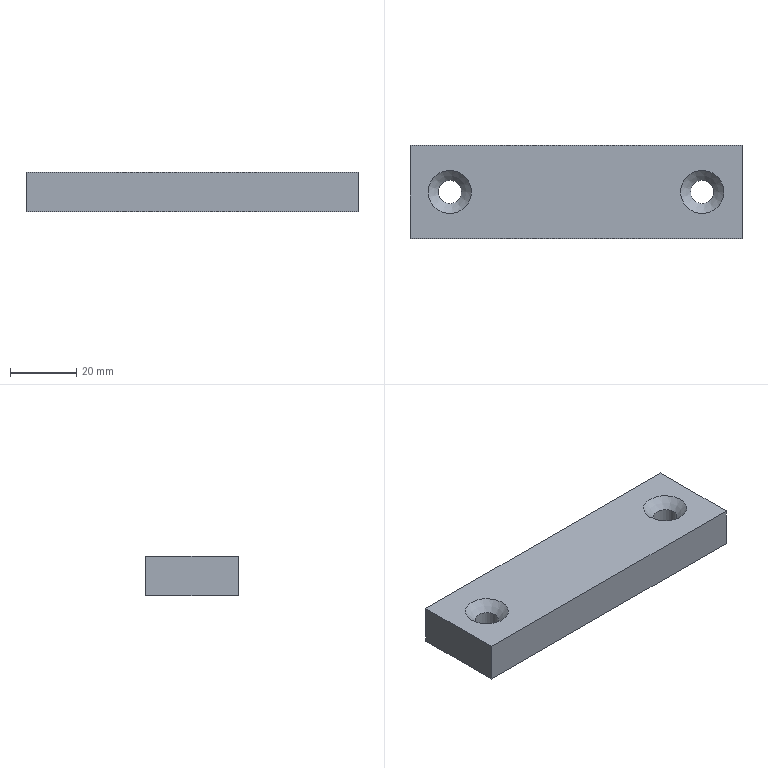Part | NX | features DATUM_CSYS 2, CHAMFER 1, EXTRUDE 1, SKETCH 1 | 1 solid | 10 faces | box 100 x 28 x 12 mm | volume 32422 mm3 | plane 6 | cylinder 2 | cone 2 | commonest cylinder face diameters 7 x2
STEP:
#1=CARTESIAN_POINT('',(-50.,-14.,0.));
#2=VERTEX_POINT('',#1);
#3=CARTESIAN_POINT('',(-50.,14.,0.));
#4=VERTEX_POINT('',#3);
#5=CARTESIAN_POINT('',(-50.,-14.,0.));
#6=DIRECTION('',(0.,1.,0.));
#7=VECTOR('',#6,1000.);
#8=LINE('',#5,#7);
#9=EDGE_CURVE('',#2,#4,#8,.T.);
#10=ORIENTED_EDGE('',*,*,#9,.T.);
#11=CARTESIAN_POINT('',(-50.,14.,-12.));
#12=VERTEX_POINT('',#11);
#13=CARTESIAN_POINT('',(-50.,14.,-12.));
#14=DIRECTION('',(0.,0.,1.));
#15=VECTOR('',#14,1000.);
#16=LINE('',#13,#15);
#17=EDGE_CURVE('',#12,#4,#16,.T.);
#18=ORIENTED_EDGE('',*,*,#17,.F.);
#19=CARTESIAN_POINT('',(-50.,-14.,-12.));
#20=VERTEX_POINT('',#19);
#21=CARTESIAN_POINT('',(-50.,-14.,-12.));
#22=DIRECTION('',(0.,1.,0.));
#23=VECTOR('',#22,1000.);
#24=LINE('',#21,#23);
#25=EDGE_CURVE('',#20,#12,#24,.T.);
#26=ORIENTED_EDGE('',*,*,#25,.F.);
#27=CARTESIAN_POINT('',(-50.,-14.,-12.));
#28=DIRECTION('',(0.,0.,1.));
#29=VECTOR('',#28,1000.);
#30=LINE('',#27,#29);
#31=EDGE_CURVE('',#20,#2,#30,.T.);
#32=ORIENTED_EDGE('',*,*,#31,.T.);
#33=EDGE_LOOP('',(#10,#18,#26,#32));
#34=FACE_BOUND('',#33,.T.);
#35=CARTESIAN_POINT('',(-50.,-14.,-12.));
#36=DIRECTION('',(1.,0.,0.));
#37=DIRECTION('',(0.,0.,-1.));
#38=AXIS2_PLACEMENT_3D('',#35,#36,#37);
#39=PLANE('',#38);
#40=ADVANCED_FACE('',(#34),#39,.F.);
#41=CARTESIAN_POINT('',(50.,14.,0.));
#42=VERTEX_POINT('',#41);
#43=CARTESIAN_POINT('',(-50.,14.,0.));
#44=DIRECTION('',(1.,0.,0.));
#45=VECTOR('',#44,1000.);
#46=LINE('',#43,#45);
#47=EDGE_CURVE('',#4,#42,#46,.T.);
#48=ORIENTED_EDGE('',*,*,#47,.T.);
#49=CARTESIAN_POINT('',(50.,14.,-12.));
#50=VERTEX_POINT('',#49);
#51=CARTESIAN_POINT('',(50.,14.,-12.));
#52=DIRECTION('',(0.,0.,1.));
#53=VECTOR('',#52,1000.);
#54=LINE('',#51,#53);
#55=EDGE_CURVE('',#50,#42,#54,.T.);
#56=ORIENTED_EDGE('',*,*,#55,.F.);
#57=CARTESIAN_POINT('',(-50.,14.,-12.));
#58=DIRECTION('',(1.,0.,0.));
#59=VECTOR('',#58,1000.);
#60=LINE('',#57,#59);
#61=EDGE_CURVE('',#12,#50,#60,.T.);
#62=ORIENTED_EDGE('',*,*,#61,.F.);
#63=ORIENTED_EDGE('',*,*,#17,.T.);
#64=EDGE_LOOP('',(#48,#56,#62,#63));
#65=FACE_BOUND('',#64,.T.);
#66=CARTESIAN_POINT('',(-50.,14.,-12.));
#67=DIRECTION('',(0.,-1.,0.));
#68=DIRECTION('',(0.,0.,-1.));
#69=AXIS2_PLACEMENT_3D('',#66,#67,#68);
#70=PLANE('',#69);
#71=ADVANCED_FACE('',(#65),#70,.F.);
#72=CARTESIAN_POINT('',(50.,-14.,0.));
#73=VERTEX_POINT('',#72);
#74=CARTESIAN_POINT('',(50.,14.,0.));
#75=DIRECTION('',(0.,-1.,0.));
#76=VECTOR('',#75,1000.);
#77=LINE('',#74,#76);
#78=EDGE_CURVE('',#42,#73,#77,.T.);
#79=ORIENTED_EDGE('',*,*,#78,.T.);
#80=CARTESIAN_POINT('',(50.,-14.,-12.));
#81=VERTEX_POINT('',#80);
#82=CARTESIAN_POINT('',(50.,-14.,-12.));
#83=DIRECTION('',(0.,0.,1.));
#84=VECTOR('',#83,1000.);
#85=LINE('',#82,#84);
#86=EDGE_CURVE('',#81,#73,#85,.T.);
#87=ORIENTED_EDGE('',*,*,#86,.F.);
#88=CARTESIAN_POINT('',(50.,14.,-12.));
#89=DIRECTION('',(0.,-1.,0.));
#90=VECTOR('',#89,1000.);
#91=LINE('',#88,#90);
#92=EDGE_CURVE('',#50,#81,#91,.T.);
#93=ORIENTED_EDGE('',*,*,#92,.F.);
#94=ORIENTED_EDGE('',*,*,#55,.T.);
#95=EDGE_LOOP('',(#79,#87,#93,#94));
#96=FACE_BOUND('',#95,.T.);
#97=CARTESIAN_POINT('',(50.,14.,-12.));
#98=DIRECTION('',(-1.,0.,0.));
#99=DIRECTION('',(0.,0.,1.));
#100=AXIS2_PLACEMENT_3D('',#97,#98,#99);
#101=PLANE('',#100);
#102=ADVANCED_FACE('',(#96),#101,.F.);
#103=CARTESIAN_POINT('',(41.5,0.,-3.));
#104=VERTEX_POINT('',#103);
#105=CARTESIAN_POINT('',(38.,0.,-3.));
#106=DIRECTION('',(0.,0.,1.));
#107=DIRECTION('',(1.,0.,0.));
#108=AXIS2_PLACEMENT_3D('',#105,#106,#107);
#109=CIRCLE('',#108,3.5);
#110=EDGE_CURVE('',#104,#104,#109,.T.);
#111=ORIENTED_EDGE('',*,*,#110,.T.);
#112=EDGE_LOOP('',(#111));
#113=FACE_BOUND('',#112,.T.);
#114=CARTESIAN_POINT('',(41.5,0.,-12.));
#115=VERTEX_POINT('',#114);
#116=CARTESIAN_POINT('',(38.,0.,-12.));
#117=DIRECTION('',(0.,0.,1.));
#118=DIRECTION('',(1.,0.,0.));
#119=AXIS2_PLACEMENT_3D('',#116,#117,#118);
#120=CIRCLE('',#119,3.5);
#121=EDGE_CURVE('',#115,#115,#120,.T.);
#122=ORIENTED_EDGE('',*,*,#121,.F.);
#123=EDGE_LOOP('',(#122));
#124=FACE_BOUND('',#123,.T.);
#125=CARTESIAN_POINT('',(38.,0.,-12.));
#126=DIRECTION('',(0.,0.,1.));
#127=DIRECTION('',(1.,0.,0.));
#128=AXIS2_PLACEMENT_3D('',#125,#126,#127);
#129=CYLINDRICAL_SURFACE('',#128,3.5);
#130=ADVANCED_FACE('',(#113,#124),#129,.F.);
#131=CARTESIAN_POINT('',(50.,-14.,0.));
#132=DIRECTION('',(-1.,0.,0.));
#133=VECTOR('',#132,1000.);
#134=LINE('',#131,#133);
#135=EDGE_CURVE('',#73,#2,#134,.T.);
#136=ORIENTED_EDGE('',*,*,#135,.T.);
#137=ORIENTED_EDGE('',*,*,#31,.F.);
#138=CARTESIAN_POINT('',(50.,-14.,-12.));
#139=DIRECTION('',(-1.,0.,0.));
#140=VECTOR('',#139,1000.);
#141=LINE('',#138,#140);
#142=EDGE_CURVE('',#81,#20,#141,.T.);
#143=ORIENTED_EDGE('',*,*,#142,.F.);
#144=ORIENTED_EDGE('',*,*,#86,.T.);
#145=EDGE_LOOP('',(#136,#137,#143,#144));
#146=FACE_BOUND('',#145,.T.);
#147=CARTESIAN_POINT('',(50.,-14.,-12.));
#148=DIRECTION('',(0.,1.,0.));
#149=DIRECTION('',(0.,0.,1.));
#150=AXIS2_PLACEMENT_3D('',#147,#148,#149);
#151=PLANE('',#150);
#152=ADVANCED_FACE('',(#146),#151,.F.);
#153=CARTESIAN_POINT('',(-34.5,0.,-3.));
#154=VERTEX_POINT('',#153);
#155=CARTESIAN_POINT('',(-38.,0.,-3.));
#156=DIRECTION('',(0.,0.,1.));
#157=DIRECTION('',(1.,0.,0.));
#158=AXIS2_PLACEMENT_3D('',#155,#156,#157);
#159=CIRCLE('',#158,3.5);
#160=EDGE_CURVE('',#154,#154,#159,.T.);
#161=ORIENTED_EDGE('',*,*,#160,.T.);
#162=EDGE_LOOP('',(#161));
#163=FACE_BOUND('',#162,.T.);
#164=CARTESIAN_POINT('',(-34.5,0.,-12.));
#165=VERTEX_POINT('',#164);
#166=CARTESIAN_POINT('',(-38.,0.,-12.));
#167=DIRECTION('',(0.,0.,1.));
#168=DIRECTION('',(1.,0.,0.));
#169=AXIS2_PLACEMENT_3D('',#166,#167,#168);
#170=CIRCLE('',#169,3.5);
#171=EDGE_CURVE('',#165,#165,#170,.T.);
#172=ORIENTED_EDGE('',*,*,#171,.F.);
#173=EDGE_LOOP('',(#172));
#174=FACE_BOUND('',#173,.T.);
#175=CARTESIAN_POINT('',(-38.,0.,-12.));
#176=DIRECTION('',(0.,0.,1.));
#177=DIRECTION('',(1.,0.,0.));
#178=AXIS2_PLACEMENT_3D('',#175,#176,#177);
#179=CYLINDRICAL_SURFACE('',#178,3.5);
#180=ADVANCED_FACE('',(#163,#174),#179,.F.);
#181=ORIENTED_EDGE('',*,*,#25,.T.);
#182=ORIENTED_EDGE('',*,*,#61,.T.);
#183=ORIENTED_EDGE('',*,*,#92,.T.);
#184=ORIENTED_EDGE('',*,*,#142,.T.);
#185=EDGE_LOOP('',(#181,#182,#183,#184));
#186=FACE_BOUND('',#185,.T.);
#187=ORIENTED_EDGE('',*,*,#121,.T.);
#188=EDGE_LOOP('',(#187));
#189=FACE_BOUND('',#188,.T.);
#190=ORIENTED_EDGE('',*,*,#171,.T.);
#191=EDGE_LOOP('',(#190));
#192=FACE_BOUND('',#191,.T.);
#193=CARTESIAN_POINT('',(38.,0.,-12.));
#194=DIRECTION('',(0.,0.,1.));
#195=DIRECTION('',(1.,0.,0.));
#196=AXIS2_PLACEMENT_3D('',#193,#194,#195);
#197=PLANE('',#196);
#198=ADVANCED_FACE('',(#186,#189,#192),#197,.F.);
#199=CARTESIAN_POINT('',(-31.5,0.,0.));
#200=VERTEX_POINT('',#199);
#201=CARTESIAN_POINT('',(-38.,0.,0.));
#202=DIRECTION('',(0.,0.,1.));
#203=DIRECTION('',(1.,0.,0.));
#204=AXIS2_PLACEMENT_3D('',#201,#202,#203);
#205=CIRCLE('',#204,6.5);
#206=EDGE_CURVE('',#200,#200,#205,.F.);
#207=ORIENTED_EDGE('',*,*,#206,.T.);
#208=EDGE_LOOP('',(#207));
#209=FACE_BOUND('',#208,.T.);
#210=CARTESIAN_POINT('',(44.5,0.,0.));
#211=VERTEX_POINT('',#210);
#212=CARTESIAN_POINT('',(38.,0.,0.));
#213=DIRECTION('',(0.,0.,1.));
#214=DIRECTION('',(1.,0.,0.));
#215=AXIS2_PLACEMENT_3D('',#212,#213,#214);
#216=CIRCLE('',#215,6.5);
#217=EDGE_CURVE('',#211,#211,#216,.F.);
#218=ORIENTED_EDGE('',*,*,#217,.T.);
#219=EDGE_LOOP('',(#218));
#220=FACE_BOUND('',#219,.T.);
#221=ORIENTED_EDGE('',*,*,#9,.F.);
#222=ORIENTED_EDGE('',*,*,#135,.F.);
#223=ORIENTED_EDGE('',*,*,#78,.F.);
#224=ORIENTED_EDGE('',*,*,#47,.F.);
#225=EDGE_LOOP('',(#221,#222,#223,#224));
#226=FACE_BOUND('',#225,.T.);
#227=CARTESIAN_POINT('',(38.,0.,0.));
#228=DIRECTION('',(0.,0.,1.));
#229=DIRECTION('',(1.,0.,0.));
#230=AXIS2_PLACEMENT_3D('',#227,#228,#229);
#231=PLANE('',#230);
#232=ADVANCED_FACE('',(#209,#220,#226),#231,.T.);
#233=ORIENTED_EDGE('',*,*,#206,.F.);
#234=EDGE_LOOP('',(#233));
#235=FACE_BOUND('',#234,.T.);
#236=ORIENTED_EDGE('',*,*,#160,.F.);
#237=EDGE_LOOP('',(#236));
#238=FACE_BOUND('',#237,.T.);
#239=CARTESIAN_POINT('',(-38.,0.,-3.));
#240=DIRECTION('',(0.,0.,1.));
#241=DIRECTION('',(1.,0.,0.));
#242=AXIS2_PLACEMENT_3D('',#239,#240,#241);
#243=CONICAL_SURFACE('',#242,3.5,0.7854);
#244=ADVANCED_FACE('',(#235,#238),#243,.F.);
#245=ORIENTED_EDGE('',*,*,#217,.F.);
#246=EDGE_LOOP('',(#245));
#247=FACE_BOUND('',#246,.T.);
#248=ORIENTED_EDGE('',*,*,#110,.F.);
#249=EDGE_LOOP('',(#248));
#250=FACE_BOUND('',#249,.T.);
#251=CARTESIAN_POINT('',(38.,0.,-3.));
#252=DIRECTION('',(0.,0.,1.));
#253=DIRECTION('',(1.,0.,0.));
#254=AXIS2_PLACEMENT_3D('',#251,#252,#253);
#255=CONICAL_SURFACE('',#254,3.5,0.7854);
#256=ADVANCED_FACE('',(#247,#250),#255,.F.);
#257=CLOSED_SHELL('',(#40,#71,#102,#130,#152,#180,#198,#232,#244,#256));
#258=MANIFOLD_SOLID_BREP('',#257);
#259=(LENGTH_UNIT()NAMED_UNIT(*)SI_UNIT(.MILLI.,.METRE.));
#260=UNCERTAINTY_MEASURE_WITH_UNIT(LENGTH_MEASURE(0.00001),#259,'','');
#261=(NAMED_UNIT(*)PLANE_ANGLE_UNIT()SI_UNIT($,.RADIAN.));
#262=(NAMED_UNIT(*)SI_UNIT($,.STERADIAN.)SOLID_ANGLE_UNIT());
#263=(GEOMETRIC_REPRESENTATION_CONTEXT(3)GLOBAL_UNCERTAINTY_ASSIGNED_CONTEXT((#260))GLOBAL_UNIT_ASSIGNED_CONTEXT((#259,#261,#262))REPRESENTATION_CONTEXT('',''));
#264=ADVANCED_BREP_SHAPE_REPRESENTATION('',(#258),#263);